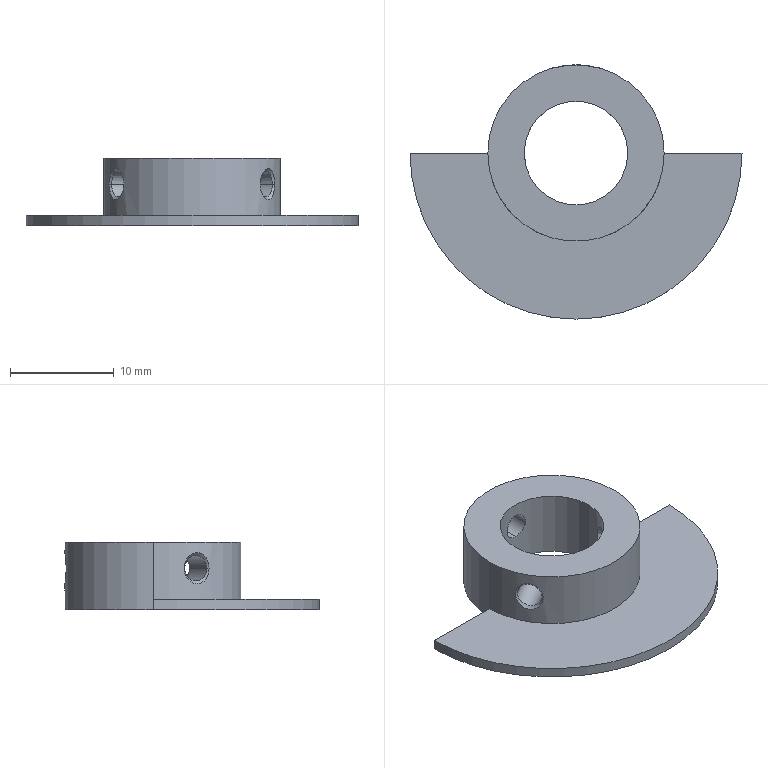Part | STEP file | 11-PSC10_psc11 | 1 solid | 30 faces | box 32 x 24.5 x 6.5 mm | volume 1203 mm3 | cone 14 | cylinder 11 | plane 5 | commonest cylinder face diameters 2.459 x6 10 x2 17 x2 32 x1
STEP:
#1=CARTESIAN_POINT('',(3.653,-3.414,4.483));
#2=VERTEX_POINT('',#1);
#3=CARTESIAN_POINT('',(3.603,-3.5,4.));
#4=VERTEX_POINT('',#3);
#5=CARTESIAN_POINT('',(4.218,-2.435,4.));
#6=DIRECTION('',(0.866,-0.5,0.));
#7=DIRECTION('',(0.5,0.866,0.));
#8=AXIS2_PLACEMENT_3D('',#5,#6,#7);
#9=CIRCLE('',#8,1.23);
#10=EDGE_CURVE('',#2,#4,#9,.T.);
#11=ORIENTED_EDGE('',*,*,#10,.T.);
#12=CARTESIAN_POINT('',(3.559,-3.512,4.));
#13=VERTEX_POINT('',#12);
#14=CARTESIAN_POINT('',(3.234,-3.599,4.));
#15=DIRECTION('',(-0.9659,-0.2588,0.));
#16=VECTOR('',#15,1000.);
#17=LINE('',#14,#16);
#18=EDGE_CURVE('',#4,#13,#17,.T.);
#19=ORIENTED_EDGE('',*,*,#18,.T.);
#20=CARTESIAN_POINT('',(3.653,-3.414,4.483));
#21=CARTESIAN_POINT('',(3.624,-3.446,4.41));
#22=CARTESIAN_POINT('',(3.6,-3.47,4.332));
#23=CARTESIAN_POINT('',(3.567,-3.503,4.168));
#24=CARTESIAN_POINT('',(3.559,-3.512,4.085));
#25=CARTESIAN_POINT('',(3.559,-3.512,4.));
#26=B_SPLINE_CURVE_WITH_KNOTS('',3,(#20,#21,#22,#23,#24,#25),.UNSPECIFIED.,.F.,.F.,(4,2,4),(0.006191,0.006444,0.006698),.UNSPECIFIED.);
#27=EDGE_CURVE('',#2,#13,#26,.T.);
#28=ORIENTED_EDGE('',*,*,#27,.F.);
#29=EDGE_LOOP('',(#11,#19,#28));
#30=FACE_OUTER_BOUND('',#29,.T.);
#31=CARTESIAN_POINT('',(3.984,-2.3,4.));
#32=DIRECTION('',(-0.866,0.5,0.));
#33=DIRECTION('',(-0.5,-0.866,0.));
#34=AXIS2_PLACEMENT_3D('',#31,#32,#33);
#35=CONICAL_SURFACE('',#34,1.5,0.7854);
#36=ADVANCED_FACE('',(#30),#35,.F.);
#37=CARTESIAN_POINT('',(3.653,-3.414,3.517));
#38=VERTEX_POINT('',#37);
#39=CARTESIAN_POINT('',(4.218,-2.435,4.));
#40=DIRECTION('',(0.866,-0.5,0.));
#41=DIRECTION('',(0.5,0.866,0.));
#42=AXIS2_PLACEMENT_3D('',#39,#40,#41);
#43=CIRCLE('',#42,1.23);
#44=EDGE_CURVE('',#4,#38,#43,.T.);
#45=ORIENTED_EDGE('',*,*,#44,.F.);
#46=CARTESIAN_POINT('',(6.512,-5.18,4.));
#47=VERTEX_POINT('',#46);
#48=CARTESIAN_POINT('',(3.369,-3.365,4.));
#49=DIRECTION('',(0.866,-0.5,0.));
#50=VECTOR('',#49,1000.);
#51=LINE('',#48,#50);
#52=EDGE_CURVE('',#4,#47,#51,.T.);
#53=ORIENTED_EDGE('',*,*,#52,.T.);
#54=CARTESIAN_POINT('',(7.742,-3.05,4.));
#55=VERTEX_POINT('',#54);
#56=CARTESIAN_POINT('',(7.127,-4.115,4.));
#57=DIRECTION('',(0.866,-0.5,0.));
#58=DIRECTION('',(0.5,0.866,0.));
#59=AXIS2_PLACEMENT_3D('',#56,#57,#58);
#60=CIRCLE('',#59,1.23);
#61=EDGE_CURVE('',#47,#55,#60,.T.);
#62=ORIENTED_EDGE('',*,*,#61,.T.);
#63=CARTESIAN_POINT('',(4.833,-1.37,4.));
#64=VERTEX_POINT('',#63);
#65=CARTESIAN_POINT('',(4.598,-1.235,4.));
#66=DIRECTION('',(0.866,-0.5,0.));
#67=VECTOR('',#66,1000.);
#68=LINE('',#65,#67);
#69=EDGE_CURVE('',#64,#55,#68,.T.);
#70=ORIENTED_EDGE('',*,*,#69,.F.);
#71=CARTESIAN_POINT('',(4.783,-1.456,3.517));
#72=VERTEX_POINT('',#71);
#73=CARTESIAN_POINT('',(4.218,-2.435,4.));
#74=DIRECTION('',(0.866,-0.5,0.));
#75=DIRECTION('',(0.5,0.866,0.));
#76=AXIS2_PLACEMENT_3D('',#73,#74,#75);
#77=CIRCLE('',#76,1.23);
#78=EDGE_CURVE('',#72,#64,#77,.T.);
#79=ORIENTED_EDGE('',*,*,#78,.F.);
#80=CARTESIAN_POINT('',(3.653,-3.414,3.517));
#81=CARTESIAN_POINT('',(3.686,-3.379,3.406));
#82=CARTESIAN_POINT('',(3.729,-3.332,3.305));
#83=CARTESIAN_POINT('',(3.831,-3.214,3.121));
#84=CARTESIAN_POINT('',(3.889,-3.144,3.041));
#85=CARTESIAN_POINT('',(4.012,-2.986,2.909));
#86=CARTESIAN_POINT('',(4.077,-2.896,2.857));
#87=CARTESIAN_POINT('',(4.206,-2.707,2.789));
#88=CARTESIAN_POINT('',(4.27,-2.604,2.771));
#89=CARTESIAN_POINT('',(4.45,-2.293,2.77));
#90=CARTESIAN_POINT('',(4.553,-2.075,2.843));
#91=CARTESIAN_POINT('',(4.705,-1.703,3.106));
#92=CARTESIAN_POINT('',(4.755,-1.549,3.295));
#93=CARTESIAN_POINT('',(4.783,-1.456,3.517));
#94=B_SPLINE_CURVE_WITH_KNOTS('',3,(#80,#81,#82,#83,#84,#85,#86,#87,#88,#89,#90,#91,#92,#93),.UNSPECIFIED.,.F.,.F.,(4,2,2,2,2,2,4),(0.,0.0003586,0.0007171,0.001076,0.001434,0.002151,0.002869),.UNSPECIFIED.);
#95=EDGE_CURVE('',#38,#72,#94,.T.);
#96=ORIENTED_EDGE('',*,*,#95,.F.);
#97=EDGE_LOOP('',(#45,#53,#62,#70,#79,#96));
#98=FACE_OUTER_BOUND('',#97,.T.);
#99=CARTESIAN_POINT('',(3.984,-2.3,4.));
#100=DIRECTION('',(0.866,-0.5,0.));
#101=DIRECTION('',(0.5,0.866,0.));
#102=AXIS2_PLACEMENT_3D('',#99,#100,#101);
#103=CYLINDRICAL_SURFACE('',#102,1.229);
#104=ADVANCED_FACE('',(#98),#103,.F.);
#105=ORIENTED_EDGE('',*,*,#61,.F.);
#106=CARTESIAN_POINT('',(6.57,-5.394,4.));
#107=VERTEX_POINT('',#106);
#108=CARTESIAN_POINT('',(6.512,-5.18,4.));
#109=DIRECTION('',(0.2588,-0.9659,0.));
#110=VECTOR('',#109,1000.);
#111=LINE('',#108,#110);
#112=EDGE_CURVE('',#47,#107,#111,.T.);
#113=ORIENTED_EDGE('',*,*,#112,.T.);
#114=CARTESIAN_POINT('',(7.956,-2.993,4.));
#115=VERTEX_POINT('',#114);
#116=CARTESIAN_POINT('',(7.956,-2.993,4.));
#117=CARTESIAN_POINT('',(7.956,-2.993,3.809));
#118=CARTESIAN_POINT('',(7.944,-3.024,3.623));
#119=CARTESIAN_POINT('',(7.896,-3.148,3.266));
#120=CARTESIAN_POINT('',(7.86,-3.239,3.103));
#121=CARTESIAN_POINT('',(7.785,-3.413,2.891));
#122=CARTESIAN_POINT('',(7.757,-3.477,2.827));
#123=CARTESIAN_POINT('',(7.694,-3.613,2.714));
#124=CARTESIAN_POINT('',(7.659,-3.688,2.664));
#125=CARTESIAN_POINT('',(7.583,-3.841,2.584));
#126=CARTESIAN_POINT('',(7.543,-3.92,2.553));
#127=CARTESIAN_POINT('',(7.456,-4.083,2.511));
#128=CARTESIAN_POINT('',(7.409,-4.167,2.5));
#129=CARTESIAN_POINT('',(7.268,-4.411,2.5));
#130=CARTESIAN_POINT('',(7.167,-4.572,2.542));
#131=CARTESIAN_POINT('',(6.977,-4.858,2.702));
#132=CARTESIAN_POINT('',(6.886,-4.985,2.821));
#133=CARTESIAN_POINT('',(6.735,-5.187,3.103));
#134=CARTESIAN_POINT('',(6.674,-5.264,3.269));
#135=CARTESIAN_POINT('',(6.591,-5.367,3.622));
#136=CARTESIAN_POINT('',(6.57,-5.394,3.812));
#137=CARTESIAN_POINT('',(6.57,-5.394,4.));
#138=B_SPLINE_CURVE_WITH_KNOTS('',3,(#116,#117,#118,#119,#120,#121,#122,#123,#124,#125,#126,#127,#128,#129,#130,#131,#132,#133,#134,#135,#136,#137),.UNSPECIFIED.,.F.,.F.,(4,2,2,2,2,2,2,2,2,2,4),(0.005795,0.006361,0.006928,0.007211,0.007494,0.007777,0.008061,0.008627,0.009193,0.00976,0.01033),.UNSPECIFIED.);
#139=EDGE_CURVE('',#115,#107,#138,.T.);
#140=ORIENTED_EDGE('',*,*,#139,.F.);
#141=CARTESIAN_POINT('',(7.742,-3.05,4.));
#142=DIRECTION('',(0.9659,0.2588,0.));
#143=VECTOR('',#142,1000.);
#144=LINE('',#141,#143);
#145=EDGE_CURVE('',#55,#115,#144,.T.);
#146=ORIENTED_EDGE('',*,*,#145,.F.);
#147=EDGE_LOOP('',(#105,#113,#140,#146));
#148=FACE_OUTER_BOUND('',#147,.T.);
#149=CARTESIAN_POINT('',(7.127,-4.115,4.));
#150=DIRECTION('',(0.866,-0.5,0.));
#151=DIRECTION('',(0.5,0.866,0.));
#152=AXIS2_PLACEMENT_3D('',#149,#150,#151);
#153=CONICAL_SURFACE('',#152,1.229,0.7854);
#154=ADVANCED_FACE('',(#148),#153,.F.);
#155=CARTESIAN_POINT('',(-4.783,-1.456,4.483));
#156=VERTEX_POINT('',#155);
#157=CARTESIAN_POINT('',(-4.833,-1.37,4.));
#158=VERTEX_POINT('',#157);
#159=CARTESIAN_POINT('',(-4.218,-2.435,4.));
#160=DIRECTION('',(-0.866,-0.5,0.));
#161=DIRECTION('',(0.5,-0.866,0.));
#162=AXIS2_PLACEMENT_3D('',#159,#160,#161);
#163=CIRCLE('',#162,1.23);
#164=EDGE_CURVE('',#156,#158,#163,.T.);
#165=ORIENTED_EDGE('',*,*,#164,.T.);
#166=CARTESIAN_POINT('',(-4.821,-1.326,4.));
#167=VERTEX_POINT('',#166);
#168=CARTESIAN_POINT('',(-4.734,-1.001,4.));
#169=DIRECTION('',(0.2588,0.9659,0.));
#170=VECTOR('',#169,1000.);
#171=LINE('',#168,#170);
#172=EDGE_CURVE('',#158,#167,#171,.T.);
#173=ORIENTED_EDGE('',*,*,#172,.T.);
#174=CARTESIAN_POINT('',(-4.783,-1.456,4.483));
#175=CARTESIAN_POINT('',(-4.796,-1.415,4.41));
#176=CARTESIAN_POINT('',(-4.805,-1.382,4.331));
#177=CARTESIAN_POINT('',(-4.818,-1.338,4.169));
#178=CARTESIAN_POINT('',(-4.821,-1.326,4.085));
#179=CARTESIAN_POINT('',(-4.821,-1.326,4.));
#180=B_SPLINE_CURVE_WITH_KNOTS('',3,(#174,#175,#176,#177,#178,#179),.UNSPECIFIED.,.F.,.F.,(4,2,4),(0.005027,0.005279,0.005531),.UNSPECIFIED.);
#181=EDGE_CURVE('',#156,#167,#180,.T.);
#182=ORIENTED_EDGE('',*,*,#181,.F.);
#183=EDGE_LOOP('',(#165,#173,#182));
#184=FACE_OUTER_BOUND('',#183,.T.);
#185=CARTESIAN_POINT('',(-3.984,-2.3,4.));
#186=DIRECTION('',(0.866,0.5,0.));
#187=DIRECTION('',(-0.5,0.866,0.));
#188=AXIS2_PLACEMENT_3D('',#185,#186,#187);
#189=CONICAL_SURFACE('',#188,1.5,0.7854);
#190=ADVANCED_FACE('',(#184),#189,.F.);
#191=CARTESIAN_POINT('',(-4.783,-1.456,3.517));
#192=VERTEX_POINT('',#191);
#193=CARTESIAN_POINT('',(-4.218,-2.435,4.));
#194=DIRECTION('',(-0.866,-0.5,0.));
#195=DIRECTION('',(0.5,-0.866,0.));
#196=AXIS2_PLACEMENT_3D('',#193,#194,#195);
#197=CIRCLE('',#196,1.23);
#198=EDGE_CURVE('',#158,#192,#197,.T.);
#199=ORIENTED_EDGE('',*,*,#198,.F.);
#200=CARTESIAN_POINT('',(-7.742,-3.05,4.));
#201=VERTEX_POINT('',#200);
#202=CARTESIAN_POINT('',(-4.598,-1.235,4.));
#203=DIRECTION('',(-0.866,-0.5,0.));
#204=VECTOR('',#203,1000.);
#205=LINE('',#202,#204);
#206=EDGE_CURVE('',#158,#201,#205,.T.);
#207=ORIENTED_EDGE('',*,*,#206,.T.);
#208=CARTESIAN_POINT('',(-6.512,-5.18,4.));
#209=VERTEX_POINT('',#208);
#210=CARTESIAN_POINT('',(-7.127,-4.115,4.));
#211=DIRECTION('',(-0.866,-0.5,0.));
#212=DIRECTION('',(0.5,-0.866,0.));
#213=AXIS2_PLACEMENT_3D('',#210,#211,#212);
#214=CIRCLE('',#213,1.229);
#215=EDGE_CURVE('',#201,#209,#214,.T.);
#216=ORIENTED_EDGE('',*,*,#215,.T.);
#217=CARTESIAN_POINT('',(-3.603,-3.5,4.));
#218=VERTEX_POINT('',#217);
#219=CARTESIAN_POINT('',(-3.369,-3.365,4.));
#220=DIRECTION('',(-0.866,-0.5,0.));
#221=VECTOR('',#220,1000.);
#222=LINE('',#219,#221);
#223=EDGE_CURVE('',#218,#209,#222,.T.);
#224=ORIENTED_EDGE('',*,*,#223,.F.);
#225=CARTESIAN_POINT('',(-3.653,-3.414,3.517));
#226=VERTEX_POINT('',#225);
#227=CARTESIAN_POINT('',(-4.218,-2.435,4.));
#228=DIRECTION('',(-0.866,-0.5,0.));
#229=DIRECTION('',(0.5,-0.866,0.));
#230=AXIS2_PLACEMENT_3D('',#227,#228,#229);
#231=CIRCLE('',#230,1.23);
#232=EDGE_CURVE('',#226,#218,#231,.T.);
#233=ORIENTED_EDGE('',*,*,#232,.F.);
#234=CARTESIAN_POINT('',(-4.783,-1.456,3.517));
#235=CARTESIAN_POINT('',(-4.769,-1.503,3.406));
#236=CARTESIAN_POINT('',(-4.75,-1.563,3.305));
#237=CARTESIAN_POINT('',(-4.699,-1.711,3.121));
#238=CARTESIAN_POINT('',(-4.667,-1.796,3.041));
#239=CARTESIAN_POINT('',(-4.592,-1.982,2.909));
#240=CARTESIAN_POINT('',(-4.547,-2.083,2.857));
#241=CARTESIAN_POINT('',(-4.447,-2.289,2.789));
#242=CARTESIAN_POINT('',(-4.39,-2.396,2.771));
#243=CARTESIAN_POINT('',(-4.211,-2.707,2.77));
#244=CARTESIAN_POINT('',(-4.074,-2.906,2.843));
#245=CARTESIAN_POINT('',(-3.828,-3.223,3.106));
#246=CARTESIAN_POINT('',(-3.719,-3.343,3.295));
#247=CARTESIAN_POINT('',(-3.653,-3.414,3.517));
#248=B_SPLINE_CURVE_WITH_KNOTS('',3,(#234,#235,#236,#237,#238,#239,#240,#241,#242,#243,#244,#245,#246,#247),.UNSPECIFIED.,.F.,.F.,(4,2,2,2,2,2,4),(0.,0.0003586,0.0007171,0.001076,0.001434,0.002151,0.002869),.UNSPECIFIED.);
#249=EDGE_CURVE('',#192,#226,#248,.T.);
#250=ORIENTED_EDGE('',*,*,#249,.F.);
#251=EDGE_LOOP('',(#199,#207,#216,#224,#233,#250));
#252=FACE_OUTER_BOUND('',#251,.T.);
#253=CARTESIAN_POINT('',(-3.984,-2.3,4.));
#254=DIRECTION('',(-0.866,-0.5,0.));
#255=DIRECTION('',(0.5,-0.866,0.));
#256=AXIS2_PLACEMENT_3D('',#253,#254,#255);
#257=CYLINDRICAL_SURFACE('',#256,1.229);
#258=ADVANCED_FACE('',(#252),#257,.F.);
#259=ORIENTED_EDGE('',*,*,#215,.F.);
#260=CARTESIAN_POINT('',(-7.956,-2.993,4.));
#261=VERTEX_POINT('',#260);
#262=CARTESIAN_POINT('',(-7.742,-3.05,4.));
#263=DIRECTION('',(-0.9659,0.2588,0.));
#264=VECTOR('',#263,1000.);
#265=LINE('',#262,#264);
#266=EDGE_CURVE('',#201,#261,#265,.T.);
#267=ORIENTED_EDGE('',*,*,#266,.T.);
#268=CARTESIAN_POINT('',(-6.57,-5.394,4.));
#269=VERTEX_POINT('',#268);
#270=CARTESIAN_POINT('',(-6.57,-5.394,4.));
#271=CARTESIAN_POINT('',(-6.57,-5.394,3.906));
#272=CARTESIAN_POINT('',(-6.575,-5.387,3.81));
#273=CARTESIAN_POINT('',(-6.596,-5.361,3.624));
#274=CARTESIAN_POINT('',(-6.612,-5.342,3.533));
#275=CARTESIAN_POINT('',(-6.653,-5.29,3.357));
#276=CARTESIAN_POINT('',(-6.679,-5.257,3.27));
#277=CARTESIAN_POINT('',(-6.739,-5.181,3.108));
#278=CARTESIAN_POINT('',(-6.773,-5.137,3.033));
#279=CARTESIAN_POINT('',(-6.848,-5.036,2.891));
#280=CARTESIAN_POINT('',(-6.89,-4.979,2.826));
#281=CARTESIAN_POINT('',(-6.977,-4.856,2.713));
#282=CARTESIAN_POINT('',(-7.022,-4.79,2.665));
#283=CARTESIAN_POINT('',(-7.166,-4.575,2.543));
#284=CARTESIAN_POINT('',(-7.267,-4.413,2.5));
#285=CARTESIAN_POINT('',(-7.455,-4.087,2.5));
#286=CARTESIAN_POINT('',(-7.544,-3.92,2.543));
#287=CARTESIAN_POINT('',(-7.696,-3.612,2.703));
#288=CARTESIAN_POINT('',(-7.76,-3.472,2.82));
#289=CARTESIAN_POINT('',(-7.835,-3.297,3.032));
#290=CARTESIAN_POINT('',(-7.856,-3.246,3.108));
#291=CARTESIAN_POINT('',(-7.893,-3.156,3.27));
#292=CARTESIAN_POINT('',(-7.908,-3.117,3.357));
#293=CARTESIAN_POINT('',(-7.944,-3.024,3.622));
#294=CARTESIAN_POINT('',(-7.956,-2.993,3.812));
#295=CARTESIAN_POINT('',(-7.956,-2.993,4.));
#296=B_SPLINE_CURVE_WITH_KNOTS('',3,(#270,#271,#272,#273,#274,#275,#276,#277,#278,#279,#280,#281,#282,#283,#284,#285,#286,#287,#288,#289,#290,#291,#292,#293,#294,#295),.UNSPECIFIED.,.F.,.F.,(4,2,2,2,2,2,2,2,2,2,2,2,4),(0.00699,0.007272,0.007554,0.007836,0.008118,0.0084,0.008683,0.009247,0.009811,0.01038,0.01066,0.01094,0.0115),.UNSPECIFIED.);
#297=EDGE_CURVE('',#269,#261,#296,.T.);
#298=ORIENTED_EDGE('',*,*,#297,.F.);
#299=CARTESIAN_POINT('',(-6.512,-5.18,4.));
#300=DIRECTION('',(-0.2588,-0.9659,0.));
#301=VECTOR('',#300,1000.);
#302=LINE('',#299,#301);
#303=EDGE_CURVE('',#209,#269,#302,.T.);
#304=ORIENTED_EDGE('',*,*,#303,.F.);
#305=EDGE_LOOP('',(#259,#267,#298,#304));
#306=FACE_OUTER_BOUND('',#305,.T.);
#307=CARTESIAN_POINT('',(-7.127,-4.115,4.));
#308=DIRECTION('',(-0.866,-0.5,0.));
#309=DIRECTION('',(0.5,-0.866,0.));
#310=AXIS2_PLACEMENT_3D('',#307,#308,#309);
#311=CONICAL_SURFACE('',#310,1.229,0.7854);
#312=ADVANCED_FACE('',(#306),#311,.F.);
#313=CARTESIAN_POINT('',(0.,5.,2.771));
#314=VERTEX_POINT('',#313);
#315=CARTESIAN_POINT('',(-1.131,4.87,3.517));
#316=VERTEX_POINT('',#315);
#317=CARTESIAN_POINT('',(0.,5.,2.771));
#318=CARTESIAN_POINT('',(-0.239,5.,2.77));
#319=CARTESIAN_POINT('',(-0.4798,4.981,2.843));
#320=CARTESIAN_POINT('',(-0.8777,4.926,3.107));
#321=CARTESIAN_POINT('',(-1.036,4.893,3.295));
#322=CARTESIAN_POINT('',(-1.131,4.87,3.517));
#323=B_SPLINE_CURVE_WITH_KNOTS('',3,(#317,#318,#319,#320,#321,#322),.UNSPECIFIED.,.F.,.F.,(4,2,4),(0.001435,0.002152,0.002869),.UNSPECIFIED.);
#324=EDGE_CURVE('',#314,#316,#323,.T.);
#325=ORIENTED_EDGE('',*,*,#324,.F.);
#326=CARTESIAN_POINT('',(0.,8.23,2.771));
#327=VERTEX_POINT('',#326);
#328=CARTESIAN_POINT('',(0.,4.6,2.771));
#329=DIRECTION('',(0.,1.,0.));
#330=VECTOR('',#329,1000.);
#331=LINE('',#328,#330);
#332=EDGE_CURVE('',#314,#327,#331,.T.);
#333=ORIENTED_EDGE('',*,*,#332,.T.);
#334=CARTESIAN_POINT('',(0.,8.23,5.229));
#335=VERTEX_POINT('',#334);
#336=CARTESIAN_POINT('',(0.,8.23,4.));
#337=DIRECTION('',(0.,1.,0.));
#338=DIRECTION('',(0.,0.,1.));
#339=AXIS2_PLACEMENT_3D('',#336,#337,#338);
#340=CIRCLE('',#339,1.229);
#341=EDGE_CURVE('',#327,#335,#340,.T.);
#342=ORIENTED_EDGE('',*,*,#341,.T.);
#343=CARTESIAN_POINT('',(0.,5.,5.229));
#344=VERTEX_POINT('',#343);
#345=CARTESIAN_POINT('',(0.,4.6,5.229));
#346=DIRECTION('',(0.,1.,0.));
#347=VECTOR('',#346,1000.);
#348=LINE('',#345,#347);
#349=EDGE_CURVE('',#344,#335,#348,.T.);
#350=ORIENTED_EDGE('',*,*,#349,.F.);
#351=CARTESIAN_POINT('',(-1.131,4.87,4.483));
#352=VERTEX_POINT('',#351);
#353=CARTESIAN_POINT('',(-1.131,4.87,4.483));
#354=CARTESIAN_POINT('',(-1.083,4.882,4.594));
#355=CARTESIAN_POINT('',(-1.021,4.895,4.695));
#356=CARTESIAN_POINT('',(-0.8679,4.925,4.879));
#357=CARTESIAN_POINT('',(-0.7782,4.94,4.959));
#358=CARTESIAN_POINT('',(-0.5796,4.967,5.091));
#359=CARTESIAN_POINT('',(-0.4694,4.979,5.143));
#360=CARTESIAN_POINT('',(-0.241,4.995,5.212));
#361=CARTESIAN_POINT('',(-0.1196,5.,5.229));
#362=CARTESIAN_POINT('',(0.,5.,5.229));
#363=B_SPLINE_CURVE_WITH_KNOTS('',3,(#353,#354,#355,#356,#357,#358,#359,#360,#361,#362),.UNSPECIFIED.,.F.,.F.,(4,2,2,2,4),(0.,0.0003587,0.0007173,0.001076,0.001435),.UNSPECIFIED.);
#364=EDGE_CURVE('',#352,#344,#363,.T.);
#365=ORIENTED_EDGE('',*,*,#364,.F.);
#366=CARTESIAN_POINT('',(0.,4.87,4.));
#367=DIRECTION('',(0.,1.,0.));
#368=DIRECTION('',(0.,0.,1.));
#369=AXIS2_PLACEMENT_3D('',#366,#367,#368);
#370=CIRCLE('',#369,1.229);
#371=EDGE_CURVE('',#316,#352,#370,.T.);
#372=ORIENTED_EDGE('',*,*,#371,.F.);
#373=EDGE_LOOP('',(#325,#333,#342,#350,#365,#372));
#374=FACE_OUTER_BOUND('',#373,.T.);
#375=CARTESIAN_POINT('',(0.,4.6,4.));
#376=DIRECTION('',(0.,1.,0.));
#377=DIRECTION('',(0.,0.,1.));
#378=AXIS2_PLACEMENT_3D('',#375,#376,#377);
#379=CYLINDRICAL_SURFACE('',#378,1.229);
#380=ADVANCED_FACE('',(#374),#379,.F.);
#381=ORIENTED_EDGE('',*,*,#341,.F.);
#382=CARTESIAN_POINT('',(0.,8.5,2.5));
#383=VERTEX_POINT('',#382);
#384=CARTESIAN_POINT('',(0.,8.23,2.771));
#385=DIRECTION('',(0.,0.7071,-0.7071));
#386=VECTOR('',#385,1000.);
#387=LINE('',#384,#386);
#388=EDGE_CURVE('',#327,#383,#387,.T.);
#389=ORIENTED_EDGE('',*,*,#388,.T.);
#390=CARTESIAN_POINT('',(0.,8.5,5.5));
#391=VERTEX_POINT('',#390);
#392=CARTESIAN_POINT('',(0.,8.5,5.5));
#393=CARTESIAN_POINT('',(-0.1899,8.5,5.5));
#394=CARTESIAN_POINT('',(-0.3789,8.493,5.457));
#395=CARTESIAN_POINT('',(-0.7213,8.471,5.296));
#396=CARTESIAN_POINT('',(-0.8747,8.456,5.179));
#397=CARTESIAN_POINT('',(-1.124,8.426,4.897));
#398=CARTESIAN_POINT('',(-1.222,8.412,4.731));
#399=CARTESIAN_POINT('',(-1.32,8.397,4.466));
#400=CARTESIAN_POINT('',(-1.345,8.393,4.373));
#401=CARTESIAN_POINT('',(-1.378,8.388,4.187));
#402=CARTESIAN_POINT('',(-1.386,8.386,4.094));
#403=CARTESIAN_POINT('',(-1.386,8.386,3.621));
#404=CARTESIAN_POINT('',(-1.25,8.411,3.244));
#405=CARTESIAN_POINT('',(-0.9348,8.449,2.889));
#406=CARTESIAN_POINT('',(-0.8657,8.456,2.825));
#407=CARTESIAN_POINT('',(-0.7151,8.47,2.712));
#408=CARTESIAN_POINT('',(-0.6329,8.477,2.662));
#409=CARTESIAN_POINT('',(-0.3777,8.493,2.543));
#410=CARTESIAN_POINT('',(-0.1881,8.5,2.5));
#411=CARTESIAN_POINT('',(0.,8.5,2.5));
#412=B_SPLINE_CURVE_WITH_KNOTS('',3,(#392,#393,#394,#395,#396,#397,#398,#399,#400,#401,#402,#403,#404,#405,#406,#407,#408,#409,#410,#411),.UNSPECIFIED.,.F.,.F.,(4,2,2,2,2,2,2,2,2,4),(0.005688,0.006254,0.00682,0.007386,0.007669,0.007952,0.009084,0.009367,0.00965,0.01022),.UNSPECIFIED.);
#413=EDGE_CURVE('',#391,#383,#412,.T.);
#414=ORIENTED_EDGE('',*,*,#413,.F.);
#415=CARTESIAN_POINT('',(0.,8.23,5.229));
#416=DIRECTION('',(0.,0.7071,0.7071));
#417=VECTOR('',#416,1000.);
#418=LINE('',#415,#417);
#419=EDGE_CURVE('',#335,#391,#418,.T.);
#420=ORIENTED_EDGE('',*,*,#419,.F.);
#421=EDGE_LOOP('',(#381,#389,#414,#420));
#422=FACE_OUTER_BOUND('',#421,.T.);
#423=CARTESIAN_POINT('',(0.,8.23,4.));
#424=DIRECTION('',(0.,1.,0.));
#425=DIRECTION('',(0.,0.,1.));
#426=AXIS2_PLACEMENT_3D('',#423,#424,#425);
#427=CONICAL_SURFACE('',#426,1.229,0.7854);
#428=ADVANCED_FACE('',(#422),#427,.F.);
#429=ORIENTED_EDGE('',*,*,#95,.T.);
#430=CARTESIAN_POINT('',(4.783,-1.456,4.483));
#431=VERTEX_POINT('',#430);
#432=CARTESIAN_POINT('',(4.783,-1.456,3.517));
#433=CARTESIAN_POINT('',(4.808,-1.375,3.662));
#434=CARTESIAN_POINT('',(4.821,-1.326,3.831));
#435=CARTESIAN_POINT('',(4.821,-1.326,4.169));
#436=CARTESIAN_POINT('',(4.808,-1.374,4.337));
#437=CARTESIAN_POINT('',(4.783,-1.456,4.483));
#438=B_SPLINE_CURVE_WITH_KNOTS('',3,(#432,#433,#434,#435,#436,#437),.UNSPECIFIED.,.F.,.F.,(4,2,4),(0.002477,0.002983,0.003488),.UNSPECIFIED.);
#439=EDGE_CURVE('',#72,#431,#438,.T.);
#440=ORIENTED_EDGE('',*,*,#439,.T.);
#441=CARTESIAN_POINT('',(4.783,-1.456,4.483));
#442=CARTESIAN_POINT('',(4.769,-1.503,4.594));
#443=CARTESIAN_POINT('',(4.75,-1.563,4.695));
#444=CARTESIAN_POINT('',(4.699,-1.711,4.879));
#445=CARTESIAN_POINT('',(4.667,-1.796,4.959));
#446=CARTESIAN_POINT('',(4.592,-1.982,5.091));
#447=CARTESIAN_POINT('',(4.547,-2.083,5.143));
#448=CARTESIAN_POINT('',(4.447,-2.289,5.211));
#449=CARTESIAN_POINT('',(4.39,-2.396,5.229));
#450=CARTESIAN_POINT('',(4.211,-2.707,5.23));
#451=CARTESIAN_POINT('',(4.074,-2.906,5.157));
#452=CARTESIAN_POINT('',(3.828,-3.223,4.894));
#453=CARTESIAN_POINT('',(3.719,-3.343,4.705));
#454=CARTESIAN_POINT('',(3.653,-3.414,4.483));
#455=B_SPLINE_CURVE_WITH_KNOTS('',3,(#441,#442,#443,#444,#445,#446,#447,#448,#449,#450,#451,#452,#453,#454),.UNSPECIFIED.,.F.,.F.,(4,2,2,2,2,2,4),(0.,0.0003586,0.0007171,0.001076,0.001434,0.002151,0.002869),.UNSPECIFIED.);
#456=EDGE_CURVE('',#431,#2,#455,.T.);
#457=ORIENTED_EDGE('',*,*,#456,.T.);
#458=ORIENTED_EDGE('',*,*,#27,.T.);
#459=CARTESIAN_POINT('',(3.559,-3.512,4.));
#460=CARTESIAN_POINT('',(3.559,-3.512,3.915));
#461=CARTESIAN_POINT('',(3.568,-3.503,3.831));
#462=CARTESIAN_POINT('',(3.6,-3.47,3.668));
#463=CARTESIAN_POINT('',(3.624,-3.446,3.59));
#464=CARTESIAN_POINT('',(3.653,-3.414,3.517));
#465=B_SPLINE_CURVE_WITH_KNOTS('',3,(#459,#460,#461,#462,#463,#464),.UNSPECIFIED.,.F.,.F.,(4,2,4),(0.006698,0.00695,0.007202),.UNSPECIFIED.);
#466=EDGE_CURVE('',#13,#38,#465,.T.);
#467=ORIENTED_EDGE('',*,*,#466,.T.);
#468=EDGE_LOOP('',(#429,#440,#457,#458,#467));
#469=FACE_BOUND('',#468,.T.);
#470=ORIENTED_EDGE('',*,*,#249,.T.);
#471=CARTESIAN_POINT('',(-3.653,-3.414,4.483));
#472=VERTEX_POINT('',#471);
#473=CARTESIAN_POINT('',(-3.653,-3.414,3.517));
#474=CARTESIAN_POINT('',(-3.623,-3.446,3.59));
#475=CARTESIAN_POINT('',(-3.6,-3.47,3.668));
#476=CARTESIAN_POINT('',(-3.568,-3.503,3.83));
#477=CARTESIAN_POINT('',(-3.559,-3.512,3.916));
#478=CARTESIAN_POINT('',(-3.559,-3.512,4.168));
#479=CARTESIAN_POINT('',(-3.594,-3.477,4.337));
#480=CARTESIAN_POINT('',(-3.653,-3.414,4.483));
#481=B_SPLINE_CURVE_WITH_KNOTS('',3,(#473,#474,#475,#476,#477,#478,#479,#480),.UNSPECIFIED.,.F.,.F.,(4,2,2,4),(0.00133,0.001582,0.001833,0.002336),.UNSPECIFIED.);
#482=EDGE_CURVE('',#226,#472,#481,.T.);
#483=ORIENTED_EDGE('',*,*,#482,.T.);
#484=CARTESIAN_POINT('',(-3.653,-3.414,4.483));
#485=CARTESIAN_POINT('',(-3.686,-3.379,4.594));
#486=CARTESIAN_POINT('',(-3.729,-3.332,4.695));
#487=CARTESIAN_POINT('',(-3.831,-3.214,4.879));
#488=CARTESIAN_POINT('',(-3.889,-3.144,4.959));
#489=CARTESIAN_POINT('',(-4.012,-2.986,5.091));
#490=CARTESIAN_POINT('',(-4.077,-2.896,5.143));
#491=CARTESIAN_POINT('',(-4.206,-2.707,5.211));
#492=CARTESIAN_POINT('',(-4.27,-2.604,5.229));
#493=CARTESIAN_POINT('',(-4.45,-2.293,5.23));
#494=CARTESIAN_POINT('',(-4.553,-2.075,5.157));
#495=CARTESIAN_POINT('',(-4.705,-1.703,4.894));
#496=CARTESIAN_POINT('',(-4.755,-1.549,4.705));
#497=CARTESIAN_POINT('',(-4.783,-1.456,4.483));
#498=B_SPLINE_CURVE_WITH_KNOTS('',3,(#484,#485,#486,#487,#488,#489,#490,#491,#492,#493,#494,#495,#496,#497),.UNSPECIFIED.,.F.,.F.,(4,2,2,2,2,2,4),(0.,0.0003586,0.0007171,0.001076,0.001434,0.002151,0.002869),.UNSPECIFIED.);
#499=EDGE_CURVE('',#472,#156,#498,.T.);
#500=ORIENTED_EDGE('',*,*,#499,.T.);
#501=ORIENTED_EDGE('',*,*,#181,.T.);
#502=CARTESIAN_POINT('',(-4.821,-1.326,4.));
#503=CARTESIAN_POINT('',(-4.821,-1.326,3.915));
#504=CARTESIAN_POINT('',(-4.818,-1.338,3.831));
#505=CARTESIAN_POINT('',(-4.805,-1.382,3.668));
#506=CARTESIAN_POINT('',(-4.796,-1.415,3.59));
#507=CARTESIAN_POINT('',(-4.783,-1.456,3.517));
#508=B_SPLINE_CURVE_WITH_KNOTS('',3,(#502,#503,#504,#505,#506,#507),.UNSPECIFIED.,.F.,.F.,(4,2,4),(0.005531,0.005782,0.006034),.UNSPECIFIED.);
#509=EDGE_CURVE('',#167,#192,#508,.T.);
#510=ORIENTED_EDGE('',*,*,#509,.T.);
#511=EDGE_LOOP('',(#470,#483,#500,#501,#510));
#512=FACE_BOUND('',#511,.T.);
#513=CARTESIAN_POINT('',(-5.,0.,6.5));
#514=VERTEX_POINT('',#513);
#515=CARTESIAN_POINT('',(5.,0.,6.5));
#516=VERTEX_POINT('',#515);
#517=CARTESIAN_POINT('',(0.,0.,6.5));
#518=DIRECTION('',(0.,0.,1.));
#519=DIRECTION('',(1.,0.,0.));
#520=AXIS2_PLACEMENT_3D('',#517,#518,#519);
#521=CIRCLE('',#520,5.);
#522=EDGE_CURVE('',#514,#516,#521,.T.);
#523=ORIENTED_EDGE('',*,*,#522,.T.);
#524=CARTESIAN_POINT('',(5.,0.,0.));
#525=VERTEX_POINT('',#524);
#526=CARTESIAN_POINT('',(5.,0.,6.5));
#527=DIRECTION('',(0.,0.,-1.));
#528=VECTOR('',#527,1000.);
#529=LINE('',#526,#528);
#530=EDGE_CURVE('',#516,#525,#529,.T.);
#531=ORIENTED_EDGE('',*,*,#530,.T.);
#532=CARTESIAN_POINT('',(-5.,0.,0.));
#533=VERTEX_POINT('',#532);
#534=CARTESIAN_POINT('',(0.,0.,0.));
#535=DIRECTION('',(0.,0.,1.));
#536=DIRECTION('',(1.,0.,0.));
#537=AXIS2_PLACEMENT_3D('',#534,#535,#536);
#538=CIRCLE('',#537,5.);
#539=EDGE_CURVE('',#533,#525,#538,.T.);
#540=ORIENTED_EDGE('',*,*,#539,.F.);
#541=CARTESIAN_POINT('',(-5.,0.,6.5));
#542=DIRECTION('',(0.,0.,-1.));
#543=VECTOR('',#542,1000.);
#544=LINE('',#541,#543);
#545=EDGE_CURVE('',#514,#533,#544,.T.);
#546=ORIENTED_EDGE('',*,*,#545,.F.);
#547=EDGE_LOOP('',(#523,#531,#540,#546));
#548=FACE_OUTER_BOUND('',#547,.T.);
#549=CARTESIAN_POINT('',(0.,0.,6.5));
#550=DIRECTION('',(0.,0.,-1.));
#551=DIRECTION('',(-1.,0.,0.));
#552=AXIS2_PLACEMENT_3D('',#549,#550,#551);
#553=CYLINDRICAL_SURFACE('',#552,5.);
#554=ADVANCED_FACE('',(#469,#512,#548),#553,.F.);
#555=ORIENTED_EDGE('',*,*,#413,.T.);
#556=CARTESIAN_POINT('',(0.,8.5,2.5));
#557=CARTESIAN_POINT('',(0.09417,8.5,2.5));
#558=CARTESIAN_POINT('',(0.1897,8.498,2.511));
#559=CARTESIAN_POINT('',(0.3745,8.492,2.552));
#560=CARTESIAN_POINT('',(0.4636,8.488,2.583));
#561=CARTESIAN_POINT('',(0.7212,8.471,2.704));
#562=CARTESIAN_POINT('',(0.8745,8.456,2.821));
#563=CARTESIAN_POINT('',(1.125,8.426,3.104));
#564=CARTESIAN_POINT('',(1.223,8.412,3.27));
#565=CARTESIAN_POINT('',(1.353,8.392,3.623));
#566=CARTESIAN_POINT('',(1.386,8.386,3.814));
#567=CARTESIAN_POINT('',(1.386,8.386,4.19));
#568=CARTESIAN_POINT('',(1.352,8.392,4.381));
#569=CARTESIAN_POINT('',(1.221,8.412,4.733));
#570=CARTESIAN_POINT('',(1.123,8.426,4.9));
#571=CARTESIAN_POINT('',(0.8735,8.456,5.18));
#572=CARTESIAN_POINT('',(0.7194,8.471,5.297));
#573=CARTESIAN_POINT('',(0.464,8.488,5.417));
#574=CARTESIAN_POINT('',(0.3728,8.492,5.448));
#575=CARTESIAN_POINT('',(0.1886,8.498,5.489));
#576=CARTESIAN_POINT('',(0.09507,8.5,5.5));
#577=CARTESIAN_POINT('',(0.,8.5,5.5));
#578=B_SPLINE_CURVE_WITH_KNOTS('',3,(#556,#557,#558,#559,#560,#561,#562,#563,#564,#565,#566,#567,#568,#569,#570,#571,#572,#573,#574,#575,#576,#577),.UNSPECIFIED.,.F.,.F.,(4,2,2,2,2,2,2,2,2,2,4),(0.001155,0.001438,0.001722,0.002288,0.002855,0.003421,0.003988,0.004555,0.005121,0.005405,0.005688),.UNSPECIFIED.);
#579=EDGE_CURVE('',#383,#391,#578,.T.);
#580=ORIENTED_EDGE('',*,*,#579,.T.);
#581=EDGE_LOOP('',(#555,#580));
#582=FACE_BOUND('',#581,.T.);
#583=CARTESIAN_POINT('',(-8.5,0.,6.5));
#584=VERTEX_POINT('',#583);
#585=CARTESIAN_POINT('',(8.5,0.,6.5));
#586=VERTEX_POINT('',#585);
#587=CARTESIAN_POINT('',(0.,0.,6.5));
#588=DIRECTION('',(0.,0.,-1.));
#589=DIRECTION('',(-1.,0.,0.));
#590=AXIS2_PLACEMENT_3D('',#587,#588,#589);
#591=CIRCLE('',#590,8.5);
#592=EDGE_CURVE('',#584,#586,#591,.T.);
#593=ORIENTED_EDGE('',*,*,#592,.T.);
#594=CARTESIAN_POINT('',(8.5,0.,1.));
#595=VERTEX_POINT('',#594);
#596=CARTESIAN_POINT('',(8.5,0.,6.5));
#597=DIRECTION('',(0.,0.,-1.));
#598=VECTOR('',#597,1000.);
#599=LINE('',#596,#598);
#600=EDGE_CURVE('',#586,#595,#599,.T.);
#601=ORIENTED_EDGE('',*,*,#600,.T.);
#602=CARTESIAN_POINT('',(8.5,0.,0.));
#603=VERTEX_POINT('',#602);
#604=CARTESIAN_POINT('',(8.5,0.,6.5));
#605=DIRECTION('',(0.,0.,-1.));
#606=VECTOR('',#605,1000.);
#607=LINE('',#604,#606);
#608=EDGE_CURVE('',#595,#603,#607,.T.);
#609=ORIENTED_EDGE('',*,*,#608,.T.);
#610=CARTESIAN_POINT('',(-8.5,0.,0.));
#611=VERTEX_POINT('',#610);
#612=CARTESIAN_POINT('',(0.,0.,0.));
#613=DIRECTION('',(0.,0.,-1.));
#614=DIRECTION('',(-1.,0.,0.));
#615=AXIS2_PLACEMENT_3D('',#612,#613,#614);
#616=CIRCLE('',#615,8.5);
#617=EDGE_CURVE('',#611,#603,#616,.T.);
#618=ORIENTED_EDGE('',*,*,#617,.F.);
#619=CARTESIAN_POINT('',(-8.5,0.,1.));
#620=VERTEX_POINT('',#619);
#621=CARTESIAN_POINT('',(-8.5,0.,6.5));
#622=DIRECTION('',(0.,0.,-1.));
#623=VECTOR('',#622,1000.);
#624=LINE('',#621,#623);
#625=EDGE_CURVE('',#620,#611,#624,.T.);
#626=ORIENTED_EDGE('',*,*,#625,.F.);
#627=CARTESIAN_POINT('',(-8.5,0.,6.5));
#628=DIRECTION('',(0.,0.,-1.));
#629=VECTOR('',#628,1000.);
#630=LINE('',#627,#629);
#631=EDGE_CURVE('',#584,#620,#630,.T.);
#632=ORIENTED_EDGE('',*,*,#631,.F.);
#633=EDGE_LOOP('',(#593,#601,#609,#618,#626,#632));
#634=FACE_OUTER_BOUND('',#633,.T.);
#635=CARTESIAN_POINT('',(0.,0.,6.5));
#636=DIRECTION('',(0.,0.,-1.));
#637=DIRECTION('',(-1.,0.,0.));
#638=AXIS2_PLACEMENT_3D('',#635,#636,#637);
#639=CYLINDRICAL_SURFACE('',#638,8.5);
#640=ADVANCED_FACE('',(#582,#634),#639,.T.);
#641=ORIENTED_EDGE('',*,*,#600,.F.);
#642=CARTESIAN_POINT('',(0.,0.,6.5));
#643=DIRECTION('',(0.,0.,-1.));
#644=DIRECTION('',(-1.,0.,0.));
#645=AXIS2_PLACEMENT_3D('',#642,#643,#644);
#646=CIRCLE('',#645,8.5);
#647=EDGE_CURVE('',#586,#584,#646,.T.);
#648=ORIENTED_EDGE('',*,*,#647,.T.);
#649=ORIENTED_EDGE('',*,*,#631,.T.);
#650=CARTESIAN_POINT('',(0.,0.,1.));
#651=DIRECTION('',(0.,0.,-1.));
#652=DIRECTION('',(-1.,0.,0.));
#653=AXIS2_PLACEMENT_3D('',#650,#651,#652);
#654=CIRCLE('',#653,8.5);
#655=EDGE_CURVE('',#595,#620,#654,.T.);
#656=ORIENTED_EDGE('',*,*,#655,.F.);
#657=EDGE_LOOP('',(#641,#648,#649,#656));
#658=FACE_OUTER_BOUND('',#657,.T.);
#659=ORIENTED_EDGE('',*,*,#297,.T.);
#660=CARTESIAN_POINT('',(-7.956,-2.993,4.));
#661=CARTESIAN_POINT('',(-7.956,-2.993,4.188));
#662=CARTESIAN_POINT('',(-7.944,-3.025,4.379));
#663=CARTESIAN_POINT('',(-7.896,-3.147,4.731));
#664=CARTESIAN_POINT('',(-7.859,-3.24,4.898));
#665=CARTESIAN_POINT('',(-7.761,-3.47,5.178));
#666=CARTESIAN_POINT('',(-7.697,-3.611,5.296));
#667=CARTESIAN_POINT('',(-7.584,-3.84,5.416));
#668=CARTESIAN_POINT('',(-7.542,-3.921,5.447));
#669=CARTESIAN_POINT('',(-7.455,-4.084,5.489));
#670=CARTESIAN_POINT('',(-7.41,-4.166,5.5));
#671=CARTESIAN_POINT('',(-7.268,-4.412,5.5));
#672=CARTESIAN_POINT('',(-7.168,-4.572,5.458));
#673=CARTESIAN_POINT('',(-6.976,-4.859,5.297));
#674=CARTESIAN_POINT('',(-6.886,-4.984,5.18));
#675=CARTESIAN_POINT('',(-6.736,-5.186,4.899));
#676=CARTESIAN_POINT('',(-6.674,-5.264,4.732));
#677=CARTESIAN_POINT('',(-6.591,-5.367,4.379));
#678=CARTESIAN_POINT('',(-6.57,-5.394,4.189));
#679=CARTESIAN_POINT('',(-6.57,-5.394,4.));
#680=B_SPLINE_CURVE_WITH_KNOTS('',3,(#660,#661,#662,#663,#664,#665,#666,#667,#668,#669,#670,#671,#672,#673,#674,#675,#676,#677,#678,#679),.UNSPECIFIED.,.F.,.F.,(4,2,2,2,2,2,2,2,2,4),(0.002472,0.003037,0.003602,0.004166,0.004449,0.004731,0.005296,0.00586,0.006425,0.00699),.UNSPECIFIED.);
#681=EDGE_CURVE('',#261,#269,#680,.T.);
#682=ORIENTED_EDGE('',*,*,#681,.T.);
#683=EDGE_LOOP('',(#659,#682));
#684=FACE_BOUND('',#683,.T.);
#685=ORIENTED_EDGE('',*,*,#139,.T.);
#686=CARTESIAN_POINT('',(6.57,-5.394,4.));
#687=CARTESIAN_POINT('',(6.57,-5.394,4.188));
#688=CARTESIAN_POINT('',(6.591,-5.367,4.378));
#689=CARTESIAN_POINT('',(6.653,-5.29,4.643));
#690=CARTESIAN_POINT('',(6.679,-5.258,4.73));
#691=CARTESIAN_POINT('',(6.739,-5.181,4.892));
#692=CARTESIAN_POINT('',(6.773,-5.137,4.967));
#693=CARTESIAN_POINT('',(6.848,-5.036,5.108));
#694=CARTESIAN_POINT('',(6.89,-4.979,5.173));
#695=CARTESIAN_POINT('',(6.977,-4.856,5.287));
#696=CARTESIAN_POINT('',(7.022,-4.79,5.335));
#697=CARTESIAN_POINT('',(7.165,-4.576,5.456));
#698=CARTESIAN_POINT('',(7.265,-4.417,5.5));
#699=CARTESIAN_POINT('',(7.408,-4.169,5.5));
#700=CARTESIAN_POINT('',(7.453,-4.087,5.49));
#701=CARTESIAN_POINT('',(7.54,-3.925,5.449));
#702=CARTESIAN_POINT('',(7.582,-3.843,5.417));
#703=CARTESIAN_POINT('',(7.696,-3.613,5.298));
#704=CARTESIAN_POINT('',(7.76,-3.472,5.18));
#705=CARTESIAN_POINT('',(7.834,-3.298,4.969));
#706=CARTESIAN_POINT('',(7.856,-3.246,4.892));
#707=CARTESIAN_POINT('',(7.893,-3.155,4.73));
#708=CARTESIAN_POINT('',(7.908,-3.117,4.645));
#709=CARTESIAN_POINT('',(7.944,-3.024,4.378));
#710=CARTESIAN_POINT('',(7.956,-2.993,4.191));
#711=CARTESIAN_POINT('',(7.956,-2.993,4.));
#712=B_SPLINE_CURVE_WITH_KNOTS('',3,(#686,#687,#688,#689,#690,#691,#692,#693,#694,#695,#696,#697,#698,#699,#700,#701,#702,#703,#704,#705,#706,#707,#708,#709,#710,#711),.UNSPECIFIED.,.F.,.F.,(4,2,2,2,2,2,2,2,2,2,2,2,4),(0.001261,0.001828,0.002111,0.002395,0.002678,0.002961,0.003528,0.003811,0.004095,0.004661,0.004945,0.005228,0.005795),.UNSPECIFIED.);
#713=EDGE_CURVE('',#107,#115,#712,.T.);
#714=ORIENTED_EDGE('',*,*,#713,.T.);
#715=EDGE_LOOP('',(#685,#714));
#716=FACE_BOUND('',#715,.T.);
#717=CARTESIAN_POINT('',(0.,0.,6.5));
#718=DIRECTION('',(0.,0.,-1.));
#719=DIRECTION('',(-1.,0.,0.));
#720=AXIS2_PLACEMENT_3D('',#717,#718,#719);
#721=CYLINDRICAL_SURFACE('',#720,8.5);
#722=ADVANCED_FACE('',(#658,#684,#716),#721,.T.);
#723=ORIENTED_EDGE('',*,*,#530,.F.);
#724=CARTESIAN_POINT('',(0.,0.,6.5));
#725=DIRECTION('',(0.,0.,1.));
#726=DIRECTION('',(1.,0.,0.));
#727=AXIS2_PLACEMENT_3D('',#724,#725,#726);
#728=CIRCLE('',#727,5.);
#729=EDGE_CURVE('',#516,#514,#728,.T.);
#730=ORIENTED_EDGE('',*,*,#729,.T.);
#731=ORIENTED_EDGE('',*,*,#545,.T.);
#732=CARTESIAN_POINT('',(0.,0.,0.));
#733=DIRECTION('',(0.,0.,1.));
#734=DIRECTION('',(1.,0.,0.));
#735=AXIS2_PLACEMENT_3D('',#732,#733,#734);
#736=CIRCLE('',#735,5.);
#737=EDGE_CURVE('',#525,#533,#736,.T.);
#738=ORIENTED_EDGE('',*,*,#737,.F.);
#739=EDGE_LOOP('',(#723,#730,#731,#738));
#740=FACE_OUTER_BOUND('',#739,.T.);
#741=ORIENTED_EDGE('',*,*,#364,.T.);
#742=CARTESIAN_POINT('',(1.131,4.87,4.483));
#743=VERTEX_POINT('',#742);
#744=CARTESIAN_POINT('',(0.,5.,5.229));
#745=CARTESIAN_POINT('',(0.239,5.,5.23));
#746=CARTESIAN_POINT('',(0.4798,4.981,5.157));
#747=CARTESIAN_POINT('',(0.8777,4.926,4.893));
#748=CARTESIAN_POINT('',(1.036,4.893,4.705));
#749=CARTESIAN_POINT('',(1.131,4.87,4.483));
#750=B_SPLINE_CURVE_WITH_KNOTS('',3,(#744,#745,#746,#747,#748,#749),.UNSPECIFIED.,.F.,.F.,(4,2,4),(0.001435,0.002152,0.002869),.UNSPECIFIED.);
#751=EDGE_CURVE('',#344,#743,#750,.T.);
#752=ORIENTED_EDGE('',*,*,#751,.T.);
#753=CARTESIAN_POINT('',(1.131,4.87,3.517));
#754=VERTEX_POINT('',#753);
#755=CARTESIAN_POINT('',(1.131,4.87,4.483));
#756=CARTESIAN_POINT('',(1.172,4.861,4.41));
#757=CARTESIAN_POINT('',(1.206,4.853,4.331));
#758=CARTESIAN_POINT('',(1.25,4.841,4.169));
#759=CARTESIAN_POINT('',(1.262,4.838,4.086));
#760=CARTESIAN_POINT('',(1.262,4.838,3.83));
#761=CARTESIAN_POINT('',(1.214,4.851,3.663));
#762=CARTESIAN_POINT('',(1.131,4.87,3.517));
#763=B_SPLINE_CURVE_WITH_KNOTS('',3,(#755,#756,#757,#758,#759,#760,#761,#762),.UNSPECIFIED.,.F.,.F.,(4,2,2,4),(0.0002162,0.0004688,0.0007215,0.001227),.UNSPECIFIED.);
#764=EDGE_CURVE('',#743,#754,#763,.T.);
#765=ORIENTED_EDGE('',*,*,#764,.T.);
#766=CARTESIAN_POINT('',(1.131,4.87,3.517));
#767=CARTESIAN_POINT('',(1.083,4.882,3.406));
#768=CARTESIAN_POINT('',(1.021,4.895,3.305));
#769=CARTESIAN_POINT('',(0.8679,4.925,3.121));
#770=CARTESIAN_POINT('',(0.7782,4.94,3.041));
#771=CARTESIAN_POINT('',(0.5796,4.967,2.909));
#772=CARTESIAN_POINT('',(0.4694,4.979,2.857));
#773=CARTESIAN_POINT('',(0.241,4.995,2.788));
#774=CARTESIAN_POINT('',(0.1196,5.,2.771));
#775=CARTESIAN_POINT('',(0.,5.,2.771));
#776=B_SPLINE_CURVE_WITH_KNOTS('',3,(#766,#767,#768,#769,#770,#771,#772,#773,#774,#775),.UNSPECIFIED.,.F.,.F.,(4,2,2,2,4),(0.,0.0003587,0.0007173,0.001076,0.001435),.UNSPECIFIED.);
#777=EDGE_CURVE('',#754,#314,#776,.T.);
#778=ORIENTED_EDGE('',*,*,#777,.T.);
#779=ORIENTED_EDGE('',*,*,#324,.T.);
#780=CARTESIAN_POINT('',(-1.131,4.87,3.517));
#781=CARTESIAN_POINT('',(-1.172,4.861,3.59));
#782=CARTESIAN_POINT('',(-1.206,4.853,3.669));
#783=CARTESIAN_POINT('',(-1.25,4.841,3.831));
#784=CARTESIAN_POINT('',(-1.262,4.838,3.914));
#785=CARTESIAN_POINT('',(-1.262,4.838,4.17));
#786=CARTESIAN_POINT('',(-1.214,4.851,4.337));
#787=CARTESIAN_POINT('',(-1.131,4.87,4.483));
#788=B_SPLINE_CURVE_WITH_KNOTS('',3,(#780,#781,#782,#783,#784,#785,#786,#787),.UNSPECIFIED.,.F.,.F.,(4,2,2,4),(0.0002162,0.0004688,0.0007215,0.001227),.UNSPECIFIED.);
#789=EDGE_CURVE('',#316,#352,#788,.T.);
#790=ORIENTED_EDGE('',*,*,#789,.T.);
#791=EDGE_LOOP('',(#741,#752,#765,#778,#779,#790));
#792=FACE_BOUND('',#791,.T.);
#793=CARTESIAN_POINT('',(0.,0.,6.5));
#794=DIRECTION('',(0.,0.,-1.));
#795=DIRECTION('',(-1.,0.,0.));
#796=AXIS2_PLACEMENT_3D('',#793,#794,#795);
#797=CYLINDRICAL_SURFACE('',#796,5.);
#798=ADVANCED_FACE('',(#740,#792),#797,.F.);
#799=CARTESIAN_POINT('',(-16.,0.,1.));
#800=VERTEX_POINT('',#799);
#801=CARTESIAN_POINT('',(16.,0.,1.));
#802=VERTEX_POINT('',#801);
#803=CARTESIAN_POINT('',(0.,0.,1.));
#804=DIRECTION('',(0.,0.,1.));
#805=DIRECTION('',(1.,0.,0.));
#806=AXIS2_PLACEMENT_3D('',#803,#804,#805);
#807=CIRCLE('',#806,16.);
#808=EDGE_CURVE('',#800,#802,#807,.T.);
#809=ORIENTED_EDGE('',*,*,#808,.F.);
#810=CARTESIAN_POINT('',(-16.,0.,0.));
#811=VERTEX_POINT('',#810);
#812=CARTESIAN_POINT('',(-16.,0.,6.5));
#813=DIRECTION('',(0.,0.,-1.));
#814=VECTOR('',#813,1000.);
#815=LINE('',#812,#814);
#816=EDGE_CURVE('',#800,#811,#815,.T.);
#817=ORIENTED_EDGE('',*,*,#816,.T.);
#818=CARTESIAN_POINT('',(16.,0.,0.));
#819=VERTEX_POINT('',#818);
#820=CARTESIAN_POINT('',(0.,0.,0.));
#821=DIRECTION('',(0.,0.,1.));
#822=DIRECTION('',(1.,0.,0.));
#823=AXIS2_PLACEMENT_3D('',#820,#821,#822);
#824=CIRCLE('',#823,16.);
#825=EDGE_CURVE('',#811,#819,#824,.T.);
#826=ORIENTED_EDGE('',*,*,#825,.T.);
#827=CARTESIAN_POINT('',(16.,0.,6.5));
#828=DIRECTION('',(0.,0.,-1.));
#829=VECTOR('',#828,1000.);
#830=LINE('',#827,#829);
#831=EDGE_CURVE('',#802,#819,#830,.T.);
#832=ORIENTED_EDGE('',*,*,#831,.F.);
#833=EDGE_LOOP('',(#809,#817,#826,#832));
#834=FACE_OUTER_BOUND('',#833,.T.);
#835=CARTESIAN_POINT('',(0.,0.,6.5));
#836=DIRECTION('',(0.,0.,-1.));
#837=DIRECTION('',(-1.,0.,0.));
#838=AXIS2_PLACEMENT_3D('',#835,#836,#837);
#839=CYLINDRICAL_SURFACE('',#838,16.);
#840=ADVANCED_FACE('',(#834),#839,.T.);
#841=ORIENTED_EDGE('',*,*,#522,.F.);
#842=ORIENTED_EDGE('',*,*,#729,.F.);
#843=EDGE_LOOP('',(#841,#842));
#844=FACE_BOUND('',#843,.T.);
#845=ORIENTED_EDGE('',*,*,#592,.F.);
#846=ORIENTED_EDGE('',*,*,#647,.F.);
#847=EDGE_LOOP('',(#845,#846));
#848=FACE_OUTER_BOUND('',#847,.T.);
#849=CARTESIAN_POINT('',(0.,0.,6.5));
#850=DIRECTION('',(0.,0.,1.));
#851=DIRECTION('',(1.,0.,0.));
#852=AXIS2_PLACEMENT_3D('',#849,#850,#851);
#853=PLANE('',#852);
#854=ADVANCED_FACE('',(#844,#848),#853,.T.);
#855=ORIENTED_EDGE('',*,*,#816,.F.);
#856=CARTESIAN_POINT('',(-8.5,0.,1.));
#857=DIRECTION('',(-1.,0.,0.));
#858=VECTOR('',#857,1000.);
#859=LINE('',#856,#858);
#860=EDGE_CURVE('',#620,#800,#859,.T.);
#861=ORIENTED_EDGE('',*,*,#860,.F.);
#862=ORIENTED_EDGE('',*,*,#625,.T.);
#863=CARTESIAN_POINT('',(-16.,0.,0.));
#864=DIRECTION('',(1.,0.,0.));
#865=VECTOR('',#864,1000.);
#866=LINE('',#863,#865);
#867=EDGE_CURVE('',#811,#611,#866,.T.);
#868=ORIENTED_EDGE('',*,*,#867,.F.);
#869=EDGE_LOOP('',(#855,#861,#862,#868));
#870=FACE_OUTER_BOUND('',#869,.T.);
#871=CARTESIAN_POINT('',(-16.,0.,6.5));
#872=DIRECTION('',(0.,1.,0.));
#873=DIRECTION('',(0.,0.,1.));
#874=AXIS2_PLACEMENT_3D('',#871,#872,#873);
#875=PLANE('',#874);
#876=ADVANCED_FACE('',(#870),#875,.T.);
#877=ORIENTED_EDGE('',*,*,#608,.F.);
#878=CARTESIAN_POINT('',(16.,0.,1.));
#879=DIRECTION('',(-1.,0.,0.));
#880=VECTOR('',#879,1000.);
#881=LINE('',#878,#880);
#882=EDGE_CURVE('',#802,#595,#881,.T.);
#883=ORIENTED_EDGE('',*,*,#882,.F.);
#884=ORIENTED_EDGE('',*,*,#831,.T.);
#885=CARTESIAN_POINT('',(8.5,0.,0.));
#886=DIRECTION('',(1.,0.,0.));
#887=VECTOR('',#886,1000.);
#888=LINE('',#885,#887);
#889=EDGE_CURVE('',#603,#819,#888,.T.);
#890=ORIENTED_EDGE('',*,*,#889,.F.);
#891=EDGE_LOOP('',(#877,#883,#884,#890));
#892=FACE_OUTER_BOUND('',#891,.T.);
#893=CARTESIAN_POINT('',(8.5,0.,6.5));
#894=DIRECTION('',(0.,1.,0.));
#895=DIRECTION('',(0.,0.,1.));
#896=AXIS2_PLACEMENT_3D('',#893,#894,#895);
#897=PLANE('',#896);
#898=ADVANCED_FACE('',(#892),#897,.T.);
#899=ORIENTED_EDGE('',*,*,#539,.T.);
#900=ORIENTED_EDGE('',*,*,#737,.T.);
#901=EDGE_LOOP('',(#899,#900));
#902=FACE_BOUND('',#901,.T.);
#903=ORIENTED_EDGE('',*,*,#867,.T.);
#904=ORIENTED_EDGE('',*,*,#617,.T.);
#905=ORIENTED_EDGE('',*,*,#889,.T.);
#906=ORIENTED_EDGE('',*,*,#825,.F.);
#907=EDGE_LOOP('',(#903,#904,#905,#906));
#908=FACE_OUTER_BOUND('',#907,.T.);
#909=CARTESIAN_POINT('',(0.,0.,0.));
#910=DIRECTION('',(0.,0.,1.));
#911=DIRECTION('',(1.,0.,0.));
#912=AXIS2_PLACEMENT_3D('',#909,#910,#911);
#913=PLANE('',#912);
#914=ADVANCED_FACE('',(#902,#908),#913,.F.);
#915=ORIENTED_EDGE('',*,*,#808,.T.);
#916=ORIENTED_EDGE('',*,*,#882,.T.);
#917=ORIENTED_EDGE('',*,*,#655,.T.);
#918=ORIENTED_EDGE('',*,*,#860,.T.);
#919=EDGE_LOOP('',(#915,#916,#917,#918));
#920=FACE_OUTER_BOUND('',#919,.T.);
#921=CARTESIAN_POINT('',(0.,0.,1.));
#922=DIRECTION('',(0.,0.,1.));
#923=DIRECTION('',(1.,0.,0.));
#924=AXIS2_PLACEMENT_3D('',#921,#922,#923);
#925=PLANE('',#924);
#926=ADVANCED_FACE('',(#920),#925,.T.);
#927=CARTESIAN_POINT('',(0.,4.87,4.));
#928=DIRECTION('',(0.,1.,0.));
#929=DIRECTION('',(0.,0.,1.));
#930=AXIS2_PLACEMENT_3D('',#927,#928,#929);
#931=CIRCLE('',#930,1.229);
#932=EDGE_CURVE('',#743,#754,#931,.T.);
#933=ORIENTED_EDGE('',*,*,#932,.T.);
#934=ORIENTED_EDGE('',*,*,#764,.F.);
#935=EDGE_LOOP('',(#933,#934));
#936=FACE_OUTER_BOUND('',#935,.T.);
#937=CARTESIAN_POINT('',(0.,4.6,4.));
#938=DIRECTION('',(0.,-1.,0.));
#939=DIRECTION('',(0.,0.,-1.));
#940=AXIS2_PLACEMENT_3D('',#937,#938,#939);
#941=CONICAL_SURFACE('',#940,1.5,0.7854);
#942=ADVANCED_FACE('',(#936),#941,.F.);
#943=ORIENTED_EDGE('',*,*,#388,.F.);
#944=CARTESIAN_POINT('',(0.,8.23,4.));
#945=DIRECTION('',(0.,1.,0.));
#946=DIRECTION('',(0.,0.,1.));
#947=AXIS2_PLACEMENT_3D('',#944,#945,#946);
#948=CIRCLE('',#947,1.229);
#949=EDGE_CURVE('',#335,#327,#948,.T.);
#950=ORIENTED_EDGE('',*,*,#949,.F.);
#951=ORIENTED_EDGE('',*,*,#419,.T.);
#952=ORIENTED_EDGE('',*,*,#579,.F.);
#953=EDGE_LOOP('',(#943,#950,#951,#952));
#954=FACE_OUTER_BOUND('',#953,.T.);
#955=CARTESIAN_POINT('',(0.,8.23,4.));
#956=DIRECTION('',(0.,1.,0.));
#957=DIRECTION('',(0.,0.,1.));
#958=AXIS2_PLACEMENT_3D('',#955,#956,#957);
#959=CONICAL_SURFACE('',#958,1.229,0.7854);
#960=ADVANCED_FACE('',(#954),#959,.F.);
#961=ORIENTED_EDGE('',*,*,#332,.F.);
#962=ORIENTED_EDGE('',*,*,#777,.F.);
#963=ORIENTED_EDGE('',*,*,#932,.F.);
#964=ORIENTED_EDGE('',*,*,#751,.F.);
#965=ORIENTED_EDGE('',*,*,#349,.T.);
#966=ORIENTED_EDGE('',*,*,#949,.T.);
#967=EDGE_LOOP('',(#961,#962,#963,#964,#965,#966));
#968=FACE_OUTER_BOUND('',#967,.T.);
#969=CARTESIAN_POINT('',(0.,4.6,4.));
#970=DIRECTION('',(0.,1.,0.));
#971=DIRECTION('',(0.,0.,1.));
#972=AXIS2_PLACEMENT_3D('',#969,#970,#971);
#973=CYLINDRICAL_SURFACE('',#972,1.229);
#974=ADVANCED_FACE('',(#968),#973,.F.);
#975=ORIENTED_EDGE('',*,*,#371,.T.);
#976=ORIENTED_EDGE('',*,*,#789,.F.);
#977=EDGE_LOOP('',(#975,#976));
#978=FACE_OUTER_BOUND('',#977,.T.);
#979=CARTESIAN_POINT('',(0.,4.6,4.));
#980=DIRECTION('',(0.,-1.,0.));
#981=DIRECTION('',(0.,0.,-1.));
#982=AXIS2_PLACEMENT_3D('',#979,#980,#981);
#983=CONICAL_SURFACE('',#982,1.5,0.7854);
#984=ADVANCED_FACE('',(#978),#983,.F.);
#985=ORIENTED_EDGE('',*,*,#232,.T.);
#986=CARTESIAN_POINT('',(-4.218,-2.435,4.));
#987=DIRECTION('',(-0.866,-0.5,0.));
#988=DIRECTION('',(0.5,-0.866,0.));
#989=AXIS2_PLACEMENT_3D('',#986,#987,#988);
#990=CIRCLE('',#989,1.23);
#991=EDGE_CURVE('',#218,#472,#990,.T.);
#992=ORIENTED_EDGE('',*,*,#991,.T.);
#993=ORIENTED_EDGE('',*,*,#482,.F.);
#994=EDGE_LOOP('',(#985,#992,#993));
#995=FACE_OUTER_BOUND('',#994,.T.);
#996=CARTESIAN_POINT('',(-3.984,-2.3,4.));
#997=DIRECTION('',(0.866,0.5,0.));
#998=DIRECTION('',(-0.5,0.866,0.));
#999=AXIS2_PLACEMENT_3D('',#996,#997,#998);
#1000=CONICAL_SURFACE('',#999,1.5,0.7854);
#1001=ADVANCED_FACE('',(#995),#1000,.F.);
#1002=ORIENTED_EDGE('',*,*,#266,.F.);
#1003=CARTESIAN_POINT('',(-7.127,-4.115,4.));
#1004=DIRECTION('',(-0.866,-0.5,0.));
#1005=DIRECTION('',(0.5,-0.866,0.));
#1006=AXIS2_PLACEMENT_3D('',#1003,#1004,#1005);
#1007=CIRCLE('',#1006,1.229);
#1008=EDGE_CURVE('',#209,#201,#1007,.T.);
#1009=ORIENTED_EDGE('',*,*,#1008,.F.);
#1010=ORIENTED_EDGE('',*,*,#303,.T.);
#1011=ORIENTED_EDGE('',*,*,#681,.F.);
#1012=EDGE_LOOP('',(#1002,#1009,#1010,#1011));
#1013=FACE_OUTER_BOUND('',#1012,.T.);
#1014=CARTESIAN_POINT('',(-7.127,-4.115,4.));
#1015=DIRECTION('',(-0.866,-0.5,0.));
#1016=DIRECTION('',(0.5,-0.866,0.));
#1017=AXIS2_PLACEMENT_3D('',#1014,#1015,#1016);
#1018=CONICAL_SURFACE('',#1017,1.229,0.7854);
#1019=ADVANCED_FACE('',(#1013),#1018,.F.);
#1020=ORIENTED_EDGE('',*,*,#206,.F.);
#1021=ORIENTED_EDGE('',*,*,#164,.F.);
#1022=ORIENTED_EDGE('',*,*,#499,.F.);
#1023=ORIENTED_EDGE('',*,*,#991,.F.);
#1024=ORIENTED_EDGE('',*,*,#223,.T.);
#1025=ORIENTED_EDGE('',*,*,#1008,.T.);
#1026=EDGE_LOOP('',(#1020,#1021,#1022,#1023,#1024,#1025));
#1027=FACE_OUTER_BOUND('',#1026,.T.);
#1028=CARTESIAN_POINT('',(-3.984,-2.3,4.));
#1029=DIRECTION('',(-0.866,-0.5,0.));
#1030=DIRECTION('',(0.5,-0.866,0.));
#1031=AXIS2_PLACEMENT_3D('',#1028,#1029,#1030);
#1032=CYLINDRICAL_SURFACE('',#1031,1.229);
#1033=ADVANCED_FACE('',(#1027),#1032,.F.);
#1034=ORIENTED_EDGE('',*,*,#172,.F.);
#1035=ORIENTED_EDGE('',*,*,#198,.T.);
#1036=ORIENTED_EDGE('',*,*,#509,.F.);
#1037=EDGE_LOOP('',(#1034,#1035,#1036));
#1038=FACE_OUTER_BOUND('',#1037,.T.);
#1039=CARTESIAN_POINT('',(-3.984,-2.3,4.));
#1040=DIRECTION('',(0.866,0.5,0.));
#1041=DIRECTION('',(-0.5,0.866,0.));
#1042=AXIS2_PLACEMENT_3D('',#1039,#1040,#1041);
#1043=CONICAL_SURFACE('',#1042,1.5,0.7854);
#1044=ADVANCED_FACE('',(#1038),#1043,.F.);
#1045=ORIENTED_EDGE('',*,*,#78,.T.);
#1046=CARTESIAN_POINT('',(4.218,-2.435,4.));
#1047=DIRECTION('',(0.866,-0.5,0.));
#1048=DIRECTION('',(0.5,0.866,0.));
#1049=AXIS2_PLACEMENT_3D('',#1046,#1047,#1048);
#1050=CIRCLE('',#1049,1.23);
#1051=EDGE_CURVE('',#64,#431,#1050,.T.);
#1052=ORIENTED_EDGE('',*,*,#1051,.T.);
#1053=ORIENTED_EDGE('',*,*,#439,.F.);
#1054=EDGE_LOOP('',(#1045,#1052,#1053));
#1055=FACE_OUTER_BOUND('',#1054,.T.);
#1056=CARTESIAN_POINT('',(3.984,-2.3,4.));
#1057=DIRECTION('',(-0.866,0.5,0.));
#1058=DIRECTION('',(-0.5,-0.866,0.));
#1059=AXIS2_PLACEMENT_3D('',#1056,#1057,#1058);
#1060=CONICAL_SURFACE('',#1059,1.5,0.7854);
#1061=ADVANCED_FACE('',(#1055),#1060,.F.);
#1062=ORIENTED_EDGE('',*,*,#112,.F.);
#1063=CARTESIAN_POINT('',(7.127,-4.115,4.));
#1064=DIRECTION('',(0.866,-0.5,0.));
#1065=DIRECTION('',(0.5,0.866,0.));
#1066=AXIS2_PLACEMENT_3D('',#1063,#1064,#1065);
#1067=CIRCLE('',#1066,1.23);
#1068=EDGE_CURVE('',#55,#47,#1067,.T.);
#1069=ORIENTED_EDGE('',*,*,#1068,.F.);
#1070=ORIENTED_EDGE('',*,*,#145,.T.);
#1071=ORIENTED_EDGE('',*,*,#713,.F.);
#1072=EDGE_LOOP('',(#1062,#1069,#1070,#1071));
#1073=FACE_OUTER_BOUND('',#1072,.T.);
#1074=CARTESIAN_POINT('',(7.127,-4.115,4.));
#1075=DIRECTION('',(0.866,-0.5,0.));
#1076=DIRECTION('',(0.5,0.866,0.));
#1077=AXIS2_PLACEMENT_3D('',#1074,#1075,#1076);
#1078=CONICAL_SURFACE('',#1077,1.229,0.7854);
#1079=ADVANCED_FACE('',(#1073),#1078,.F.);
#1080=ORIENTED_EDGE('',*,*,#52,.F.);
#1081=ORIENTED_EDGE('',*,*,#10,.F.);
#1082=ORIENTED_EDGE('',*,*,#456,.F.);
#1083=ORIENTED_EDGE('',*,*,#1051,.F.);
#1084=ORIENTED_EDGE('',*,*,#69,.T.);
#1085=ORIENTED_EDGE('',*,*,#1068,.T.);
#1086=EDGE_LOOP('',(#1080,#1081,#1082,#1083,#1084,#1085));
#1087=FACE_OUTER_BOUND('',#1086,.T.);
#1088=CARTESIAN_POINT('',(3.984,-2.3,4.));
#1089=DIRECTION('',(0.866,-0.5,0.));
#1090=DIRECTION('',(0.5,0.866,0.));
#1091=AXIS2_PLACEMENT_3D('',#1088,#1089,#1090);
#1092=CYLINDRICAL_SURFACE('',#1091,1.229);
#1093=ADVANCED_FACE('',(#1087),#1092,.F.);
#1094=ORIENTED_EDGE('',*,*,#18,.F.);
#1095=ORIENTED_EDGE('',*,*,#44,.T.);
#1096=ORIENTED_EDGE('',*,*,#466,.F.);
#1097=EDGE_LOOP('',(#1094,#1095,#1096));
#1098=FACE_OUTER_BOUND('',#1097,.T.);
#1099=CARTESIAN_POINT('',(3.984,-2.3,4.));
#1100=DIRECTION('',(-0.866,0.5,0.));
#1101=DIRECTION('',(-0.5,-0.866,0.));
#1102=AXIS2_PLACEMENT_3D('',#1099,#1100,#1101);
#1103=CONICAL_SURFACE('',#1102,1.5,0.7854);
#1104=ADVANCED_FACE('',(#1098),#1103,.F.);
#1105=CLOSED_SHELL('',(#36,#104,#154,#190,#258,#312,#380,#428,#554,#640,#722,#798,#840,#854,#876,#898,#914,#926,#942,#960,#974,#984,#1001,#1019,#1033,#1044,#1061,#1079,#1093,#1104));
#1106=MANIFOLD_SOLID_BREP('',#1105);
#1107=CARTESIAN_POINT('',(0.,0.,0.));
#1108=DIRECTION('',(0.,0.,1.));
#1109=DIRECTION('',(1.,0.,0.));
#1110=AXIS2_PLACEMENT_3D('',#1107,#1108,#1109);
#1111=(LENGTH_UNIT()NAMED_UNIT(*)SI_UNIT(.MILLI.,.METRE.));
#1112=UNCERTAINTY_MEASURE_WITH_UNIT(LENGTH_MEASURE(0.00001),#1111,'','');
#1113=(NAMED_UNIT(*)PLANE_ANGLE_UNIT()SI_UNIT($,.RADIAN.));
#1114=(NAMED_UNIT(*)SI_UNIT($,.STERADIAN.)SOLID_ANGLE_UNIT());
#1115=(GEOMETRIC_REPRESENTATION_CONTEXT(3)GLOBAL_UNCERTAINTY_ASSIGNED_CONTEXT((#1112))GLOBAL_UNIT_ASSIGNED_CONTEXT((#1111,#1113,#1114))REPRESENTATION_CONTEXT('',''));
#1116=ADVANCED_BREP_SHAPE_REPRESENTATION('',(#1106,#1110),#1115);